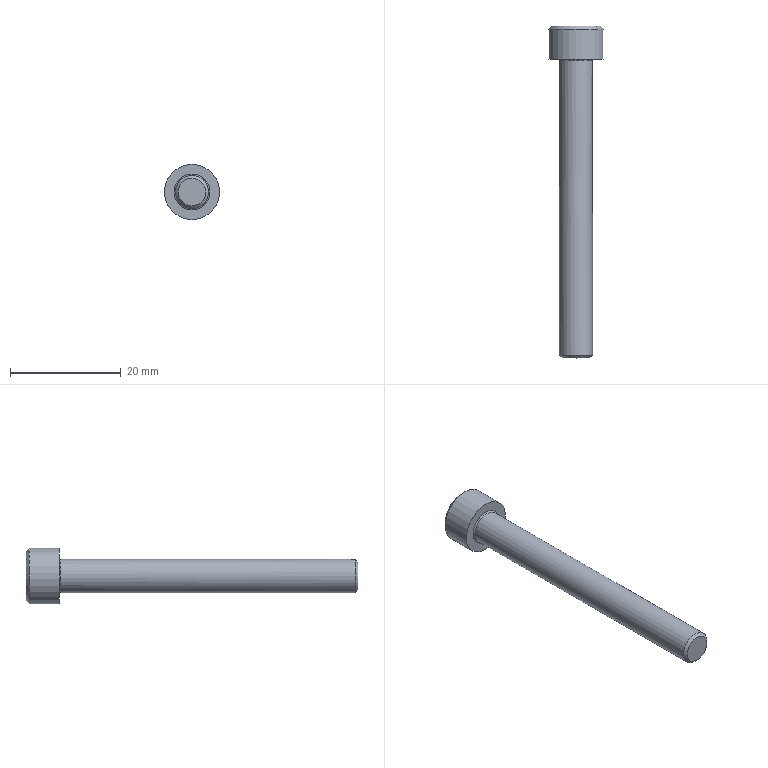Part | STEP file | solid 53 | 1 solid | 21 faces | box 10 x 60 x 10 mm | volume 1925 mm3 | plane 10 | sphere 6 | cylinder 2 | cone 2 | torus 1 | commonest cylinder face diameters 6 x1 10 x1